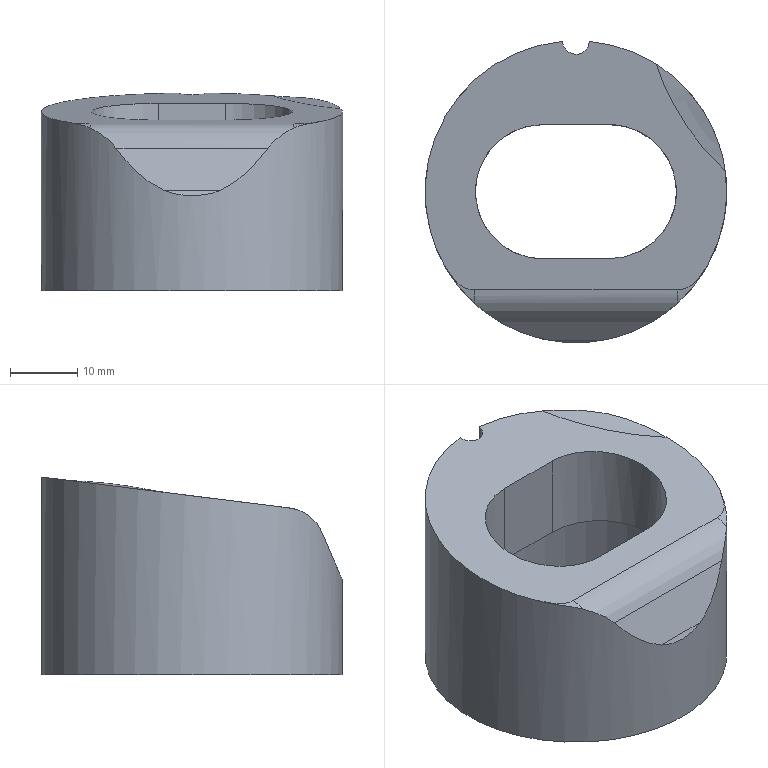Part | NX | features solid 2 | 1 solid | 18 faces | box 45 x 44.911 x 29.533 mm | volume 20669 mm3 | cylinder 9 | plane 6 | spline 3 | commonest cylinder face diameters 11.998 x2 20 x2 4 x1 12 x1 15 x1 36 x1
STEP:
#1=CARTESIAN_POINT('',(325.175,-191.134,24.41));
#2=VERTEX_POINT('',#1);
#3=CARTESIAN_POINT('',(325.178,-191.138,24.409));
#4=VERTEX_POINT('',#3);
#5=CARTESIAN_POINT('',(325.175,-191.134,24.41));
#6=CARTESIAN_POINT('',(325.176,-191.136,24.41));
#7=CARTESIAN_POINT('',(325.177,-191.137,24.41));
#8=CARTESIAN_POINT('',(325.178,-191.138,24.41));
#9=B_SPLINE_CURVE_WITH_KNOTS('',3,(#5,#6,#7,#8),.UNSPECIFIED.,.F.,.F.,(4,4),(0.6136,0.6142),.UNSPECIFIED.);
#10=EDGE_CURVE('',#2,#4,#9,.T.);
#11=ORIENTED_EDGE('',*,*,#10,.F.);
#12=CARTESIAN_POINT('',(343.002,-158.081,28.533));
#13=VERTEX_POINT('',#12);
#14=CARTESIAN_POINT('',(345.,-180.493,25.738));
#15=DIRECTION('',(0.,-0.1238,0.9923));
#16=DIRECTION('',(0.,0.9923,0.1238));
#17=AXIS2_PLACEMENT_3D('',#14,#15,#16);
#18=ELLIPSE('',#17,22.674,22.5);
#19=EDGE_CURVE('',#13,#2,#18,.T.);
#20=ORIENTED_EDGE('',*,*,#19,.F.);
#21=CARTESIAN_POINT('',(343.002,-158.081,-1.));
#22=VERTEX_POINT('',#21);
#23=CARTESIAN_POINT('',(343.002,-158.081,14.));
#24=DIRECTION('',(0.,0.,-1.));
#25=VECTOR('',#24,1000.);
#26=LINE('',#23,#25);
#27=EDGE_CURVE('',#22,#13,#26,.F.);
#28=ORIENTED_EDGE('',*,*,#27,.F.);
#29=CARTESIAN_POINT('',(346.998,-158.081,-1.));
#30=VERTEX_POINT('',#29);
#31=CARTESIAN_POINT('',(345.,-180.493,-1.));
#32=DIRECTION('',(0.,0.,-1.));
#33=DIRECTION('',(-1.,0.,0.));
#34=AXIS2_PLACEMENT_3D('',#31,#32,#33);
#35=CIRCLE('',#34,22.5);
#36=EDGE_CURVE('',#30,#22,#35,.T.);
#37=ORIENTED_EDGE('',*,*,#36,.F.);
#38=CARTESIAN_POINT('',(346.998,-158.081,28.533));
#39=VERTEX_POINT('',#38);
#40=CARTESIAN_POINT('',(346.998,-158.081,14.));
#41=DIRECTION('',(0.,0.,-1.));
#42=VECTOR('',#41,1000.);
#43=LINE('',#40,#42);
#44=EDGE_CURVE('',#39,#30,#43,.T.);
#45=ORIENTED_EDGE('',*,*,#44,.F.);
#46=CARTESIAN_POINT('',(357.006,-161.463,28.111));
#47=VERTEX_POINT('',#46);
#48=CARTESIAN_POINT('',(345.,-180.493,25.738));
#49=DIRECTION('',(0.,-0.1238,0.9923));
#50=DIRECTION('',(0.,0.9923,0.1238));
#51=AXIS2_PLACEMENT_3D('',#48,#49,#50);
#52=ELLIPSE('',#51,22.674,22.5);
#53=EDGE_CURVE('',#47,#39,#52,.T.);
#54=ORIENTED_EDGE('',*,*,#53,.F.);
#55=CARTESIAN_POINT('',(367.291,-177.436,26.119));
#56=VERTEX_POINT('',#55);
#57=CARTESIAN_POINT('',(367.291,-177.435,26.119));
#58=CARTESIAN_POINT('',(367.068,-175.804,26.322));
#59=CARTESIAN_POINT('',(366.286,-172.681,26.923));
#60=CARTESIAN_POINT('',(363.366,-166.778,27.871));
#61=CARTESIAN_POINT('',(359.804,-163.229,27.891));
#62=CARTESIAN_POINT('',(357.006,-161.463,28.111));
#63=B_SPLINE_CURVE_WITH_KNOTS('',3,(#57,#58,#59,#60,#61,#62),.UNSPECIFIED.,.F.,.F.,(4,1,1,4),(0.,0.004909,0.009818,0.01964),.UNSPECIFIED.);
#64=EDGE_CURVE('',#56,#47,#63,.T.);
#65=ORIENTED_EDGE('',*,*,#64,.F.);
#66=CARTESIAN_POINT('',(364.825,-191.134,24.41));
#67=VERTEX_POINT('',#66);
#68=CARTESIAN_POINT('',(345.,-180.493,25.738));
#69=DIRECTION('',(0.,-0.1238,0.9923));
#70=DIRECTION('',(0.,0.9923,0.1238));
#71=AXIS2_PLACEMENT_3D('',#68,#69,#70);
#72=ELLIPSE('',#71,22.674,22.5);
#73=EDGE_CURVE('',#67,#56,#72,.T.);
#74=ORIENTED_EDGE('',*,*,#73,.F.);
#75=CARTESIAN_POINT('',(364.822,-191.138,24.409));
#76=VERTEX_POINT('',#75);
#77=CARTESIAN_POINT('',(364.822,-191.138,24.41));
#78=CARTESIAN_POINT('',(364.823,-191.136,24.41));
#79=CARTESIAN_POINT('',(364.824,-191.135,24.41));
#80=CARTESIAN_POINT('',(364.825,-191.134,24.41));
#81=B_SPLINE_CURVE_WITH_KNOTS('',3,(#77,#78,#79,#80),.UNSPECIFIED.,.F.,.F.,(4,4),(0.3858,0.3865),.UNSPECIFIED.);
#82=EDGE_CURVE('',#76,#67,#81,.T.);
#83=ORIENTED_EDGE('',*,*,#82,.F.);
#84=CARTESIAN_POINT('',(363.388,-193.46,24.118));
#85=VERTEX_POINT('',#84);
#86=CARTESIAN_POINT('',(364.822,-191.138,24.409));
#87=CARTESIAN_POINT('',(364.392,-191.94,24.309));
#88=CARTESIAN_POINT('',(363.913,-192.714,24.211));
#89=CARTESIAN_POINT('',(363.388,-193.46,24.118));
#90=B_SPLINE_CURVE_WITH_KNOTS('',3,(#86,#87,#88,#89),.UNSPECIFIED.,.F.,.F.,(4,4),(0.0003971,0.003142),.UNSPECIFIED.);
#91=EDGE_CURVE('',#76,#85,#90,.T.);
#92=ORIENTED_EDGE('',*,*,#91,.T.);
#93=CARTESIAN_POINT('',(360.131,-197.145,23.293));
#94=VERTEX_POINT('',#93);
#95=CARTESIAN_POINT('',(363.388,-193.46,24.119));
#96=CARTESIAN_POINT('',(362.429,-194.818,23.95));
#97=CARTESIAN_POINT('',(361.302,-196.081,23.84));
#98=CARTESIAN_POINT('',(360.131,-197.145,23.293));
#99=B_SPLINE_CURVE_WITH_KNOTS('',3,(#95,#96,#97,#98),.UNSPECIFIED.,.F.,.F.,(4,4),(0.,0.005011),.UNSPECIFIED.);
#100=EDGE_CURVE('',#85,#94,#99,.T.);
#101=ORIENTED_EDGE('',*,*,#100,.T.);
#102=CARTESIAN_POINT('',(356.336,-199.928,20.3));
#103=VERTEX_POINT('',#102);
#104=CARTESIAN_POINT('',(360.131,-197.145,23.293));
#105=CARTESIAN_POINT('',(359.468,-197.747,22.984));
#106=CARTESIAN_POINT('',(358.149,-198.805,22.193));
#107=CARTESIAN_POINT('',(356.866,-199.619,21.027));
#108=CARTESIAN_POINT('',(356.336,-199.928,20.3));
#109=B_SPLINE_CURVE_WITH_KNOTS('',3,(#104,#105,#106,#107,#108),.UNSPECIFIED.,.F.,.F.,(4,1,4),(0.,0.002803,0.005605),.UNSPECIFIED.);
#110=EDGE_CURVE('',#94,#103,#109,.T.);
#111=ORIENTED_EDGE('',*,*,#110,.T.);
#112=CARTESIAN_POINT('',(349.112,-202.614,13.973));
#113=VERTEX_POINT('',#112);
#114=CARTESIAN_POINT('',(345.,-180.493,66.089));
#115=DIRECTION('',(0.,0.9205,-0.3907));
#116=DIRECTION('',(0.,0.3907,0.9205));
#117=AXIS2_PLACEMENT_3D('',#114,#115,#116);
#118=ELLIPSE('',#117,57.586,22.5);
#119=EDGE_CURVE('',#113,#103,#118,.F.);
#120=ORIENTED_EDGE('',*,*,#119,.F.);
#121=CARTESIAN_POINT('',(340.888,-202.614,13.973));
#122=VERTEX_POINT('',#121);
#123=CARTESIAN_POINT('',(340.888,-202.614,13.973));
#124=CARTESIAN_POINT('',(342.176,-202.853,13.409));
#125=CARTESIAN_POINT('',(344.991,-203.132,13.001));
#126=CARTESIAN_POINT('',(347.826,-202.853,13.41));
#127=CARTESIAN_POINT('',(349.112,-202.614,13.973));
#128=B_SPLINE_CURVE_WITH_KNOTS('',3,(#123,#124,#125,#126,#127),.UNSPECIFIED.,.F.,.F.,(4,1,4),(0.,0.004206,0.008413),.UNSPECIFIED.);
#129=EDGE_CURVE('',#122,#113,#128,.T.);
#130=ORIENTED_EDGE('',*,*,#129,.F.);
#131=CARTESIAN_POINT('',(333.664,-199.928,20.3));
#132=VERTEX_POINT('',#131);
#133=CARTESIAN_POINT('',(345.,-180.493,66.089));
#134=DIRECTION('',(0.,0.9205,-0.3907));
#135=DIRECTION('',(0.,0.3907,0.9205));
#136=AXIS2_PLACEMENT_3D('',#133,#134,#135);
#137=ELLIPSE('',#136,57.586,22.5);
#138=EDGE_CURVE('',#132,#122,#137,.F.);
#139=ORIENTED_EDGE('',*,*,#138,.F.);
#140=CARTESIAN_POINT('',(329.869,-197.145,23.293));
#141=VERTEX_POINT('',#140);
#142=CARTESIAN_POINT('',(333.664,-199.928,20.3));
#143=CARTESIAN_POINT('',(332.603,-199.309,21.757));
#144=CARTESIAN_POINT('',(331.194,-198.348,22.676));
#145=CARTESIAN_POINT('',(329.869,-197.145,23.293));
#146=B_SPLINE_CURVE_WITH_KNOTS('',3,(#142,#143,#144,#145),.UNSPECIFIED.,.F.,.F.,(4,4),(0.,0.00561),.UNSPECIFIED.);
#147=EDGE_CURVE('',#132,#141,#146,.T.);
#148=ORIENTED_EDGE('',*,*,#147,.T.);
#149=CARTESIAN_POINT('',(326.612,-193.46,24.119));
#150=VERTEX_POINT('',#149);
#151=CARTESIAN_POINT('',(329.869,-197.145,23.293));
#152=CARTESIAN_POINT('',(328.699,-196.082,23.839));
#153=CARTESIAN_POINT('',(327.57,-194.818,23.95));
#154=CARTESIAN_POINT('',(326.612,-193.46,24.119));
#155=B_SPLINE_CURVE_WITH_KNOTS('',3,(#151,#152,#153,#154),.UNSPECIFIED.,.F.,.F.,(4,4),(0.,0.005002),.UNSPECIFIED.);
#156=EDGE_CURVE('',#141,#150,#155,.T.);
#157=ORIENTED_EDGE('',*,*,#156,.T.);
#158=CARTESIAN_POINT('',(326.612,-193.46,24.119));
#159=CARTESIAN_POINT('',(326.087,-192.714,24.211));
#160=CARTESIAN_POINT('',(325.609,-191.94,24.309));
#161=CARTESIAN_POINT('',(325.178,-191.138,24.409));
#162=B_SPLINE_CURVE_WITH_KNOTS('',3,(#158,#159,#160,#161),.UNSPECIFIED.,.F.,.F.,(4,4),(0.0000426,0.002787),.UNSPECIFIED.);
#163=EDGE_CURVE('',#150,#4,#162,.T.);
#164=ORIENTED_EDGE('',*,*,#163,.T.);
#165=EDGE_LOOP('',(#11,#20,#28,#37,#45,#54,#65,#74,#83,#92,#101,#111,#120,#130,#139,#148,#157,#164));
#166=FACE_BOUND('',#165,.T.);
#167=CARTESIAN_POINT('',(345.,-180.493,-1.));
#168=DIRECTION('',(0.,0.,1.));
#169=DIRECTION('',(-1.,0.,0.));
#170=AXIS2_PLACEMENT_3D('',#167,#168,#169);
#171=CYLINDRICAL_SURFACE('',#170,22.5);
#172=ADVANCED_FACE('',(#166),#171,.T.);
#173=CARTESIAN_POINT('',(340.,-190.493,14.));
#174=VERTEX_POINT('',#173);
#175=CARTESIAN_POINT('',(340.,-190.493,24.49));
#176=VERTEX_POINT('',#175);
#177=CARTESIAN_POINT('',(340.,-190.493,-251.));
#178=DIRECTION('',(0.,0.,1.));
#179=VECTOR('',#178,1000.);
#180=LINE('',#177,#179);
#181=EDGE_CURVE('',#174,#176,#180,.T.);
#182=ORIENTED_EDGE('',*,*,#181,.T.);
#183=CARTESIAN_POINT('',(350.,-190.493,24.49));
#184=VERTEX_POINT('',#183);
#185=CARTESIAN_POINT('',(340.,-190.493,24.49));
#186=DIRECTION('',(1.,0.,0.));
#187=VECTOR('',#186,1000.);
#188=LINE('',#185,#187);
#189=EDGE_CURVE('',#176,#184,#188,.T.);
#190=ORIENTED_EDGE('',*,*,#189,.T.);
#191=CARTESIAN_POINT('',(350.,-190.493,14.));
#192=VERTEX_POINT('',#191);
#193=CARTESIAN_POINT('',(350.,-190.493,-251.));
#194=DIRECTION('',(0.,0.,1.));
#195=VECTOR('',#194,1000.);
#196=LINE('',#193,#195);
#197=EDGE_CURVE('',#192,#184,#196,.T.);
#198=ORIENTED_EDGE('',*,*,#197,.F.);
#199=CARTESIAN_POINT('',(340.,-190.493,14.));
#200=DIRECTION('',(-1.,0.,0.));
#201=VECTOR('',#200,1000.);
#202=LINE('',#199,#201);
#203=EDGE_CURVE('',#192,#174,#202,.T.);
#204=ORIENTED_EDGE('',*,*,#203,.T.);
#205=EDGE_LOOP('',(#182,#190,#198,#204));
#206=FACE_BOUND('',#205,.T.);
#207=CARTESIAN_POINT('',(340.,-190.493,-251.));
#208=DIRECTION('',(0.,1.,0.));
#209=DIRECTION('',(0.,0.,1.));
#210=AXIS2_PLACEMENT_3D('',#207,#208,#209);
#211=PLANE('',#210);
#212=ADVANCED_FACE('',(#206),#211,.T.);
#213=CARTESIAN_POINT('',(359.96,-181.391,25.625));
#214=VERTEX_POINT('',#213);
#215=CARTESIAN_POINT('',(350.,-180.493,25.738));
#216=DIRECTION('',(0.,-0.1238,0.9923));
#217=DIRECTION('',(0.,0.9923,0.1238));
#218=AXIS2_PLACEMENT_3D('',#215,#216,#217);
#219=ELLIPSE('',#218,10.078,10.);
#220=EDGE_CURVE('',#214,#184,#219,.F.);
#221=ORIENTED_EDGE('',*,*,#220,.F.);
#222=CARTESIAN_POINT('',(359.958,-179.573,25.852));
#223=VERTEX_POINT('',#222);
#224=CARTESIAN_POINT('',(359.958,-179.573,25.852));
#225=CARTESIAN_POINT('',(360.014,-180.18,25.777));
#226=CARTESIAN_POINT('',(360.014,-180.789,25.701));
#227=CARTESIAN_POINT('',(359.96,-181.391,25.625));
#228=B_SPLINE_CURVE_WITH_KNOTS('',3,(#224,#225,#226,#227),.UNSPECIFIED.,.F.,.F.,(4,4),(0.4706,0.5289),.UNSPECIFIED.);
#229=EDGE_CURVE('',#223,#214,#228,.T.);
#230=ORIENTED_EDGE('',*,*,#229,.F.);
#231=CARTESIAN_POINT('',(350.,-170.493,26.985));
#232=VERTEX_POINT('',#231);
#233=CARTESIAN_POINT('',(350.,-180.493,25.738));
#234=DIRECTION('',(0.,-0.1238,0.9923));
#235=DIRECTION('',(0.,0.9923,0.1238));
#236=AXIS2_PLACEMENT_3D('',#233,#234,#235);
#237=ELLIPSE('',#236,10.078,10.);
#238=EDGE_CURVE('',#232,#223,#237,.F.);
#239=ORIENTED_EDGE('',*,*,#238,.F.);
#240=CARTESIAN_POINT('',(350.,-170.493,14.));
#241=VERTEX_POINT('',#240);
#242=CARTESIAN_POINT('',(350.,-170.493,-251.));
#243=DIRECTION('',(0.,0.,1.));
#244=VECTOR('',#243,1000.);
#245=LINE('',#242,#244);
#246=EDGE_CURVE('',#241,#232,#245,.T.);
#247=ORIENTED_EDGE('',*,*,#246,.F.);
#248=CARTESIAN_POINT('',(350.,-180.493,14.));
#249=DIRECTION('',(0.,0.,-1.));
#250=DIRECTION('',(-1.,0.,0.));
#251=AXIS2_PLACEMENT_3D('',#248,#249,#250);
#252=CIRCLE('',#251,10.);
#253=EDGE_CURVE('',#192,#241,#252,.F.);
#254=ORIENTED_EDGE('',*,*,#253,.F.);
#255=ORIENTED_EDGE('',*,*,#197,.T.);
#256=EDGE_LOOP('',(#221,#230,#239,#247,#254,#255));
#257=FACE_BOUND('',#256,.T.);
#258=CARTESIAN_POINT('',(350.,-180.493,-251.));
#259=DIRECTION('',(0.,0.,1.));
#260=DIRECTION('',(-1.,0.,0.));
#261=AXIS2_PLACEMENT_3D('',#258,#259,#260);
#262=CYLINDRICAL_SURFACE('',#261,10.);
#263=ADVANCED_FACE('',(#257),#262,.F.);
#264=CARTESIAN_POINT('',(340.,-170.493,26.985));
#265=VERTEX_POINT('',#264);
#266=CARTESIAN_POINT('',(340.,-170.493,26.985));
#267=DIRECTION('',(1.,0.,0.));
#268=VECTOR('',#267,1000.);
#269=LINE('',#266,#268);
#270=EDGE_CURVE('',#265,#232,#269,.T.);
#271=ORIENTED_EDGE('',*,*,#270,.F.);
#272=CARTESIAN_POINT('',(340.,-170.493,14.));
#273=VERTEX_POINT('',#272);
#274=CARTESIAN_POINT('',(340.,-170.493,-251.));
#275=DIRECTION('',(0.,0.,1.));
#276=VECTOR('',#275,1000.);
#277=LINE('',#274,#276);
#278=EDGE_CURVE('',#273,#265,#277,.T.);
#279=ORIENTED_EDGE('',*,*,#278,.F.);
#280=CARTESIAN_POINT('',(340.,-170.493,14.));
#281=DIRECTION('',(-1.,0.,0.));
#282=VECTOR('',#281,1000.);
#283=LINE('',#280,#282);
#284=EDGE_CURVE('',#241,#273,#283,.T.);
#285=ORIENTED_EDGE('',*,*,#284,.F.);
#286=ORIENTED_EDGE('',*,*,#246,.T.);
#287=EDGE_LOOP('',(#271,#279,#285,#286));
#288=FACE_BOUND('',#287,.T.);
#289=CARTESIAN_POINT('',(340.,-170.493,-251.));
#290=DIRECTION('',(0.,1.,0.));
#291=DIRECTION('',(0.,0.,1.));
#292=AXIS2_PLACEMENT_3D('',#289,#290,#291);
#293=PLANE('',#292);
#294=ADVANCED_FACE('',(#288),#293,.F.);
#295=CARTESIAN_POINT('',(330.042,-181.411,25.623));
#296=VERTEX_POINT('',#295);
#297=CARTESIAN_POINT('',(340.,-180.493,25.738));
#298=DIRECTION('',(0.,-0.1238,0.9923));
#299=DIRECTION('',(0.,0.9923,0.1238));
#300=AXIS2_PLACEMENT_3D('',#297,#298,#299);
#301=ELLIPSE('',#300,10.078,10.);
#302=EDGE_CURVE('',#176,#296,#301,.F.);
#303=ORIENTED_EDGE('',*,*,#302,.F.);
#304=ORIENTED_EDGE('',*,*,#181,.F.);
#305=CARTESIAN_POINT('',(340.,-180.493,14.));
#306=DIRECTION('',(0.,0.,-1.));
#307=DIRECTION('',(-1.,0.,0.));
#308=AXIS2_PLACEMENT_3D('',#305,#306,#307);
#309=CIRCLE('',#308,10.);
#310=EDGE_CURVE('',#273,#174,#309,.F.);
#311=ORIENTED_EDGE('',*,*,#310,.F.);
#312=ORIENTED_EDGE('',*,*,#278,.T.);
#313=CARTESIAN_POINT('',(330.04,-179.594,25.85));
#314=VERTEX_POINT('',#313);
#315=CARTESIAN_POINT('',(340.,-180.493,25.738));
#316=DIRECTION('',(0.,-0.1238,0.9923));
#317=DIRECTION('',(0.,0.9923,0.1238));
#318=AXIS2_PLACEMENT_3D('',#315,#316,#317);
#319=ELLIPSE('',#318,10.078,10.);
#320=EDGE_CURVE('',#314,#265,#319,.F.);
#321=ORIENTED_EDGE('',*,*,#320,.F.);
#322=CARTESIAN_POINT('',(330.042,-181.411,25.623));
#323=CARTESIAN_POINT('',(329.986,-180.804,25.699));
#324=CARTESIAN_POINT('',(329.986,-180.196,25.775));
#325=CARTESIAN_POINT('',(330.04,-179.594,25.85));
#326=B_SPLINE_CURVE_WITH_KNOTS('',3,(#322,#323,#324,#325),.UNSPECIFIED.,.F.,.F.,(4,4),(0.4706,0.5289),.UNSPECIFIED.);
#327=EDGE_CURVE('',#296,#314,#326,.T.);
#328=ORIENTED_EDGE('',*,*,#327,.F.);
#329=EDGE_LOOP('',(#303,#304,#311,#312,#321,#328));
#330=FACE_BOUND('',#329,.T.);
#331=CARTESIAN_POINT('',(340.,-180.493,-251.));
#332=DIRECTION('',(0.,0.,1.));
#333=DIRECTION('',(-1.,0.,0.));
#334=AXIS2_PLACEMENT_3D('',#331,#332,#333);
#335=CYLINDRICAL_SURFACE('',#334,10.);
#336=ADVANCED_FACE('',(#330),#335,.F.);
#337=CARTESIAN_POINT('',(345.,-157.993,28.544));
#338=DIRECTION('',(0.,-0.1238,0.9923));
#339=DIRECTION('',(0.,-0.9923,-0.1238));
#340=AXIS2_PLACEMENT_3D('',#337,#338,#339);
#341=ELLIPSE('',#340,2.016,2.);
#342=EDGE_CURVE('',#39,#13,#341,.F.);
#343=ORIENTED_EDGE('',*,*,#342,.F.);
#344=ORIENTED_EDGE('',*,*,#44,.T.);
#345=CARTESIAN_POINT('',(345.,-157.993,-1.));
#346=DIRECTION('',(0.,0.,-1.));
#347=DIRECTION('',(0.,-1.,0.));
#348=AXIS2_PLACEMENT_3D('',#345,#346,#347);
#349=CIRCLE('',#348,2.);
#350=EDGE_CURVE('',#30,#22,#349,.T.);
#351=ORIENTED_EDGE('',*,*,#350,.T.);
#352=ORIENTED_EDGE('',*,*,#27,.T.);
#353=EDGE_LOOP('',(#343,#344,#351,#352));
#354=FACE_BOUND('',#353,.T.);
#355=CARTESIAN_POINT('',(345.,-157.993,29.));
#356=DIRECTION('',(0.,0.,-1.));
#357=DIRECTION('',(0.,1.,0.));
#358=AXIS2_PLACEMENT_3D('',#355,#356,#357);
#359=CYLINDRICAL_SURFACE('',#358,2.);
#360=ADVANCED_FACE('',(#354),#359,.F.);
#361=ORIENTED_EDGE('',*,*,#36,.T.);
#362=ORIENTED_EDGE('',*,*,#350,.F.);
#363=EDGE_LOOP('',(#361,#362));
#364=FACE_BOUND('',#363,.T.);
#365=CARTESIAN_POINT('',(327.,-180.493,-1.));
#366=VERTEX_POINT('',#365);
#367=CARTESIAN_POINT('',(345.,-180.493,-1.));
#368=DIRECTION('',(0.,0.,-1.));
#369=DIRECTION('',(-1.,0.,0.));
#370=AXIS2_PLACEMENT_3D('',#367,#368,#369);
#371=CIRCLE('',#370,18.);
#372=EDGE_CURVE('',#366,#366,#371,.F.);
#373=ORIENTED_EDGE('',*,*,#372,.T.);
#374=EDGE_LOOP('',(#373));
#375=FACE_BOUND('',#374,.T.);
#376=CARTESIAN_POINT('',(345.,-180.493,-1.));
#377=DIRECTION('',(0.,0.,1.));
#378=DIRECTION('',(-1.,0.,0.));
#379=AXIS2_PLACEMENT_3D('',#376,#377,#378);
#380=PLANE('',#379);
#381=ADVANCED_FACE('',(#364,#375),#380,.F.);
#382=CARTESIAN_POINT('',(327.,-180.493,14.));
#383=VERTEX_POINT('',#382);
#384=CARTESIAN_POINT('',(345.,-180.493,14.));
#385=DIRECTION('',(0.,0.,-1.));
#386=DIRECTION('',(-1.,0.,0.));
#387=AXIS2_PLACEMENT_3D('',#384,#385,#386);
#388=CIRCLE('',#387,18.);
#389=EDGE_CURVE('',#383,#383,#388,.T.);
#390=ORIENTED_EDGE('',*,*,#389,.F.);
#391=EDGE_LOOP('',(#390));
#392=FACE_BOUND('',#391,.T.);
#393=ORIENTED_EDGE('',*,*,#372,.F.);
#394=EDGE_LOOP('',(#393));
#395=FACE_BOUND('',#394,.T.);
#396=CARTESIAN_POINT('',(345.,-180.493,21.));
#397=DIRECTION('',(0.,0.,-1.));
#398=DIRECTION('',(1.,0.,0.));
#399=AXIS2_PLACEMENT_3D('',#396,#397,#398);
#400=CYLINDRICAL_SURFACE('',#399,18.);
#401=ADVANCED_FACE('',(#392,#395),#400,.F.);
#402=ORIENTED_EDGE('',*,*,#203,.F.);
#403=ORIENTED_EDGE('',*,*,#253,.T.);
#404=ORIENTED_EDGE('',*,*,#284,.T.);
#405=ORIENTED_EDGE('',*,*,#310,.T.);
#406=EDGE_LOOP('',(#402,#403,#404,#405));
#407=FACE_BOUND('',#406,.T.);
#408=ORIENTED_EDGE('',*,*,#389,.T.);
#409=EDGE_LOOP('',(#408));
#410=FACE_BOUND('',#409,.T.);
#411=CARTESIAN_POINT('',(345.,-180.493,14.));
#412=DIRECTION('',(0.,0.,1.));
#413=DIRECTION('',(-1.,0.,0.));
#414=AXIS2_PLACEMENT_3D('',#411,#412,#413);
#415=PLANE('',#414);
#416=ADVANCED_FACE('',(#407,#410),#415,.F.);
#417=ORIENTED_EDGE('',*,*,#73,.T.);
#418=CARTESIAN_POINT('',(367.29,-177.439,26.119));
#419=CARTESIAN_POINT('',(362.583,-173.071,26.663));
#420=CARTESIAN_POINT('',(358.98,-167.562,27.351));
#421=CARTESIAN_POINT('',(357.004,-161.463,28.111));
#422=B_SPLINE_CURVE_WITH_KNOTS('',3,(#418,#419,#420,#421),.UNSPECIFIED.,.F.,.F.,(4,4),(0.1646,0.5757),.UNSPECIFIED.);
#423=EDGE_CURVE('',#56,#47,#422,.T.);
#424=ORIENTED_EDGE('',*,*,#423,.T.);
#425=ORIENTED_EDGE('',*,*,#53,.T.);
#426=ORIENTED_EDGE('',*,*,#342,.T.);
#427=ORIENTED_EDGE('',*,*,#19,.T.);
#428=ORIENTED_EDGE('',*,*,#10,.T.);
#429=CARTESIAN_POINT('',(326.718,-193.389,24.129));
#430=VERTEX_POINT('',#429);
#431=CARTESIAN_POINT('',(325.178,-191.138,24.41));
#432=CARTESIAN_POINT('',(325.691,-191.888,24.316));
#433=CARTESIAN_POINT('',(326.205,-192.639,24.222));
#434=CARTESIAN_POINT('',(326.718,-193.389,24.129));
#435=B_SPLINE_CURVE_WITH_KNOTS('',3,(#431,#432,#433,#434),.UNSPECIFIED.,.F.,.F.,(4,4),(0.6142,1.),.UNSPECIFIED.);
#436=EDGE_CURVE('',#4,#430,#435,.T.);
#437=ORIENTED_EDGE('',*,*,#436,.T.);
#438=CARTESIAN_POINT('',(329.869,-195.148,23.909));
#439=VERTEX_POINT('',#438);
#440=CARTESIAN_POINT('',(326.718,-193.389,24.129));
#441=CARTESIAN_POINT('',(326.837,-193.558,24.108));
#442=CARTESIAN_POINT('',(326.981,-193.748,24.084));
#443=CARTESIAN_POINT('',(327.433,-194.232,24.024));
#444=CARTESIAN_POINT('',(328.051,-194.689,23.967));
#445=CARTESIAN_POINT('',(328.787,-195.002,23.928));
#446=CARTESIAN_POINT('',(329.314,-195.113,23.914));
#447=CARTESIAN_POINT('',(329.645,-195.141,23.91));
#448=CARTESIAN_POINT('',(329.764,-195.145,23.91));
#449=CARTESIAN_POINT('',(329.869,-195.148,23.909));
#450=B_SPLINE_CURVE_WITH_KNOTS('',3,(#440,#441,#442,#443,#444,#445,#446,#447,#448,#449),.UNSPECIFIED.,.F.,.F.,(4,1,1,1,1,1,1,4),(0.,0.125,0.25,0.5,0.75,0.875,0.9375,1.),.UNSPECIFIED.);
#451=EDGE_CURVE('',#430,#439,#450,.T.);
#452=ORIENTED_EDGE('',*,*,#451,.T.);
#453=CARTESIAN_POINT('',(360.131,-195.148,23.909));
#454=VERTEX_POINT('',#453);
#455=CARTESIAN_POINT('',(329.869,-195.148,23.909));
#456=CARTESIAN_POINT('',(339.956,-195.148,23.909));
#457=CARTESIAN_POINT('',(350.044,-195.148,23.909));
#458=CARTESIAN_POINT('',(360.131,-195.148,23.909));
#459=B_SPLINE_CURVE_WITH_KNOTS('',3,(#455,#456,#457,#458),.UNSPECIFIED.,.F.,.F.,(4,4),(0.,1.),.UNSPECIFIED.);
#460=EDGE_CURVE('',#439,#454,#459,.T.);
#461=ORIENTED_EDGE('',*,*,#460,.T.);
#462=CARTESIAN_POINT('',(363.281,-193.389,24.129));
#463=VERTEX_POINT('',#462);
#464=CARTESIAN_POINT('',(360.131,-195.148,23.909));
#465=CARTESIAN_POINT('',(360.339,-195.145,23.91));
#466=CARTESIAN_POINT('',(360.578,-195.129,23.912));
#467=CARTESIAN_POINT('',(361.23,-195.003,23.927));
#468=CARTESIAN_POINT('',(361.942,-194.69,23.966));
#469=CARTESIAN_POINT('',(362.566,-194.233,24.023));
#470=CARTESIAN_POINT('',(363.019,-193.75,24.084));
#471=CARTESIAN_POINT('',(363.159,-193.56,24.107));
#472=CARTESIAN_POINT('',(363.281,-193.39,24.129));
#473=B_SPLINE_CURVE_WITH_KNOTS('',3,(#464,#465,#466,#467,#468,#469,#470,#471,#472),.UNSPECIFIED.,.F.,.F.,(4,1,1,1,1,1,4),(0.,0.125,0.25,0.5,0.75,0.875,1.),.UNSPECIFIED.);
#474=EDGE_CURVE('',#454,#463,#473,.T.);
#475=ORIENTED_EDGE('',*,*,#474,.T.);
#476=CARTESIAN_POINT('',(363.282,-193.389,24.129));
#477=CARTESIAN_POINT('',(363.795,-192.638,24.222));
#478=CARTESIAN_POINT('',(364.309,-191.888,24.316));
#479=CARTESIAN_POINT('',(364.822,-191.138,24.41));
#480=B_SPLINE_CURVE_WITH_KNOTS('',3,(#476,#477,#478,#479),.UNSPECIFIED.,.F.,.F.,(4,4),(0.,0.3858),.UNSPECIFIED.);
#481=EDGE_CURVE('',#463,#76,#480,.T.);
#482=ORIENTED_EDGE('',*,*,#481,.T.);
#483=ORIENTED_EDGE('',*,*,#82,.T.);
#484=EDGE_LOOP('',(#417,#424,#425,#426,#427,#428,#437,#452,#461,#475,#482,#483));
#485=FACE_BOUND('',#484,.T.);
#486=ORIENTED_EDGE('',*,*,#229,.T.);
#487=ORIENTED_EDGE('',*,*,#220,.T.);
#488=ORIENTED_EDGE('',*,*,#189,.F.);
#489=ORIENTED_EDGE('',*,*,#302,.T.);
#490=ORIENTED_EDGE('',*,*,#327,.T.);
#491=ORIENTED_EDGE('',*,*,#320,.T.);
#492=ORIENTED_EDGE('',*,*,#270,.T.);
#493=ORIENTED_EDGE('',*,*,#238,.T.);
#494=EDGE_LOOP('',(#486,#487,#488,#489,#490,#491,#492,#493));
#495=FACE_BOUND('',#494,.T.);
#496=CARTESIAN_POINT('',(300.,-92.289,36.741));
#497=DIRECTION('',(0.,-0.1238,0.9923));
#498=DIRECTION('',(0.,0.9923,0.1238));
#499=AXIS2_PLACEMENT_3D('',#496,#497,#498);
#500=PLANE('',#499);
#501=ADVANCED_FACE('',(#485,#495),#500,.T.);
#502=CARTESIAN_POINT('',(349.112,-202.614,13.973));
#503=CARTESIAN_POINT('',(346.371,-202.614,13.973));
#504=CARTESIAN_POINT('',(343.629,-202.614,13.973));
#505=CARTESIAN_POINT('',(340.888,-202.614,13.973));
#506=B_SPLINE_CURVE_WITH_KNOTS('',3,(#502,#503,#504,#505),.UNSPECIFIED.,.F.,.F.,(4,4),(0.364,0.636),.UNSPECIFIED.);
#507=EDGE_CURVE('',#113,#122,#506,.T.);
#508=ORIENTED_EDGE('',*,*,#507,.T.);
#509=ORIENTED_EDGE('',*,*,#129,.T.);
#510=EDGE_LOOP('',(#508,#509));
#511=FACE_BOUND('',#510,.T.);
#512=CARTESIAN_POINT('',(354.069,-209.517,16.904));
#513=DIRECTION('',(1.,0.,0.));
#514=DIRECTION('',(0.,1.,0.));
#515=AXIS2_PLACEMENT_3D('',#512,#513,#514);
#516=CYLINDRICAL_SURFACE('',#515,7.5);
#517=ADVANCED_FACE('',(#511),#516,.F.);
#518=CARTESIAN_POINT('',(333.664,-199.928,20.3));
#519=CARTESIAN_POINT('',(341.221,-199.928,20.3));
#520=CARTESIAN_POINT('',(348.779,-199.928,20.3));
#521=CARTESIAN_POINT('',(356.336,-199.928,20.3));
#522=B_SPLINE_CURVE_WITH_KNOTS('',3,(#518,#519,#520,#521),.UNSPECIFIED.,.F.,.F.,(4,4),(0.1254,0.8746),.UNSPECIFIED.);
#523=EDGE_CURVE('',#132,#103,#522,.T.);
#524=ORIENTED_EDGE('',*,*,#523,.F.);
#525=ORIENTED_EDGE('',*,*,#138,.T.);
#526=ORIENTED_EDGE('',*,*,#507,.F.);
#527=ORIENTED_EDGE('',*,*,#119,.T.);
#528=EDGE_LOOP('',(#524,#525,#526,#527));
#529=FACE_BOUND('',#528,.T.);
#530=CARTESIAN_POINT('',(360.312,-199.928,20.3));
#531=DIRECTION('',(0.,0.9205,-0.3907));
#532=DIRECTION('',(0.,-0.3907,-0.9205));
#533=AXIS2_PLACEMENT_3D('',#530,#531,#532);
#534=PLANE('',#533);
#535=ADVANCED_FACE('',(#529),#534,.F.);
#536=ORIENTED_EDGE('',*,*,#423,.F.);
#537=ORIENTED_EDGE('',*,*,#64,.T.);
#538=EDGE_LOOP('',(#536,#537));
#539=FACE_BOUND('',#538,.T.);
#540=CARTESIAN_POINT('',(370.014,-175.954,26.616));
#541=CARTESIAN_POINT('',(368.713,-174.589,26.802));
#542=CARTESIAN_POINT('',(367.472,-173.09,27.004));
#543=CARTESIAN_POINT('',(365.774,-170.65,27.329));
#544=CARTESIAN_POINT('',(365.244,-169.821,27.439));
#545=CARTESIAN_POINT('',(364.24,-168.096,27.667));
#546=CARTESIAN_POINT('',(363.737,-167.132,27.794));
#547=CARTESIAN_POINT('',(362.629,-164.805,28.099));
#548=CARTESIAN_POINT('',(361.893,-162.979,28.337));
#549=CARTESIAN_POINT('',(361.269,-160.795,28.619));
#550=CARTESIAN_POINT('',(361.257,-160.756,28.624));
#551=CARTESIAN_POINT('',(361.246,-160.717,28.63));
#552=CARTESIAN_POINT('',(368.706,-176.704,26.21));
#553=CARTESIAN_POINT('',(367.301,-175.326,26.382));
#554=CARTESIAN_POINT('',(365.955,-173.8,26.572));
#555=CARTESIAN_POINT('',(364.106,-171.299,26.884));
#556=CARTESIAN_POINT('',(363.527,-170.446,26.991));
#557=CARTESIAN_POINT('',(362.428,-168.667,27.213));
#558=CARTESIAN_POINT('',(361.877,-167.669,27.337));
#559=CARTESIAN_POINT('',(360.659,-165.256,27.638));
#560=CARTESIAN_POINT('',(359.846,-163.358,27.875));
#561=CARTESIAN_POINT('',(359.151,-161.078,28.159));
#562=CARTESIAN_POINT('',(359.138,-161.038,28.165));
#563=CARTESIAN_POINT('',(359.126,-160.997,28.17));
#564=CARTESIAN_POINT('',(367.372,-177.509,26.11));
#565=CARTESIAN_POINT('',(365.861,-176.119,26.283));
#566=CARTESIAN_POINT('',(364.408,-174.568,26.477));
#567=CARTESIAN_POINT('',(362.404,-172.005,26.796));
#568=CARTESIAN_POINT('',(361.776,-171.13,26.906));
#569=CARTESIAN_POINT('',(360.581,-169.296,27.134));
#570=CARTESIAN_POINT('',(359.981,-168.266,27.263));
#571=CARTESIAN_POINT('',(358.651,-165.767,27.574));
#572=CARTESIAN_POINT('',(357.76,-163.796,27.82));
#573=CARTESIAN_POINT('',(356.992,-161.42,28.117));
#574=CARTESIAN_POINT('',(356.978,-161.378,28.122));
#575=CARTESIAN_POINT('',(356.965,-161.335,28.127));
#576=(BOUNDED_SURFACE()B_SPLINE_SURFACE(2,3,((#540,#541,#542,#543,#544,#545,#546,#547,#548,#549,#550,#551),(#552,#553,#554,#555,#556,#557,#558,#559,#560,#561,#562,#563),(#564,#565,#566,#567,#568,#569,#570,#571,#572,#573,#574,#575)),.UNSPECIFIED.,.F.,.F.,.F.)B_SPLINE_SURFACE_WITH_KNOTS((3,3),(4,2,2,2,2,4),(0.8161,1.),(0.5603,0.625,0.6562,0.6875,0.75,0.7511),.UNSPECIFIED.)GEOMETRIC_REPRESENTATION_ITEM()RATIONAL_B_SPLINE_SURFACE(((0.9544,0.9548,0.9552,0.9557,0.9558,0.9562,0.9563,0.9567,0.9569,0.9571,0.9571,0.9571),(0.9721,0.9723,0.9725,0.9729,0.973,0.9731,0.9732,0.9734,0.9736,0.9737,0.9737,0.9737),(1.,1.,1.,1.,1.,1.,1.,1.,1.,1.,1.,1.)))REPRESENTATION_ITEM('')SURFACE());
#577=ADVANCED_FACE('',(#539),#576,.F.);
#578=ORIENTED_EDGE('',*,*,#163,.F.);
#579=CARTESIAN_POINT('',(326.612,-193.46,24.119));
#580=CARTESIAN_POINT('',(326.648,-193.436,24.122));
#581=CARTESIAN_POINT('',(326.683,-193.413,24.126));
#582=CARTESIAN_POINT('',(326.718,-193.389,24.129));
#583=B_SPLINE_CURVE_WITH_KNOTS('',3,(#579,#580,#581,#582),.UNSPECIFIED.,.F.,.F.,(4,4),(0.9881,1.),.UNSPECIFIED.);
#584=EDGE_CURVE('',#430,#150,#583,.F.);
#585=ORIENTED_EDGE('',*,*,#584,.F.);
#586=ORIENTED_EDGE('',*,*,#436,.F.);
#587=EDGE_LOOP('',(#578,#585,#586));
#588=FACE_BOUND('',#587,.T.);
#589=CARTESIAN_POINT('',(325.92,-191.479,18.322));
#590=DIRECTION('',(0.5619,-0.8208,-0.1023));
#591=DIRECTION('',(0.8252,0.5649,0.));
#592=AXIS2_PLACEMENT_3D('',#589,#590,#591);
#593=CYLINDRICAL_SURFACE('',#592,5.999);
#594=ADVANCED_FACE('',(#588),#593,.T.);
#595=ORIENTED_EDGE('',*,*,#156,.F.);
#596=CARTESIAN_POINT('',(329.869,-195.148,23.909));
#597=CARTESIAN_POINT('',(329.869,-195.843,23.823));
#598=CARTESIAN_POINT('',(329.869,-196.522,23.613));
#599=CARTESIAN_POINT('',(329.869,-197.145,23.293));
#600=B_SPLINE_CURVE_WITH_KNOTS('',3,(#596,#597,#598,#599),.UNSPECIFIED.,.F.,.F.,(4,4),(0.,0.335),.UNSPECIFIED.);
#601=EDGE_CURVE('',#439,#141,#600,.T.);
#602=ORIENTED_EDGE('',*,*,#601,.F.);
#603=ORIENTED_EDGE('',*,*,#451,.F.);
#604=ORIENTED_EDGE('',*,*,#584,.T.);
#605=EDGE_LOOP('',(#595,#602,#603,#604));
#606=FACE_BOUND('',#605,.T.);
#607=CARTESIAN_POINT('',(329.869,-195.148,23.909));
#608=CARTESIAN_POINT('',(329.869,-196.208,23.777));
#609=CARTESIAN_POINT('',(329.869,-197.157,23.287));
#610=CARTESIAN_POINT('',(329.552,-195.148,23.909));
#611=CARTESIAN_POINT('',(329.455,-196.208,23.777));
#612=CARTESIAN_POINT('',(329.363,-197.157,23.287));
#613=CARTESIAN_POINT('',(329.243,-195.105,23.915));
#614=CARTESIAN_POINT('',(329.05,-196.158,23.783));
#615=CARTESIAN_POINT('',(328.869,-197.099,23.291));
#616=CARTESIAN_POINT('',(328.866,-195.002,23.928));
#617=CARTESIAN_POINT('',(328.554,-196.036,23.799));
#618=CARTESIAN_POINT('',(328.262,-196.957,23.299));
#619=CARTESIAN_POINT('',(328.791,-194.979,23.93));
#620=CARTESIAN_POINT('',(328.455,-196.008,23.802));
#621=CARTESIAN_POINT('',(328.141,-196.925,23.301));
#622=CARTESIAN_POINT('',(328.642,-194.927,23.937));
#623=CARTESIAN_POINT('',(328.259,-195.948,23.81));
#624=CARTESIAN_POINT('',(327.901,-196.854,23.305));
#625=CARTESIAN_POINT('',(328.568,-194.899,23.94));
#626=CARTESIAN_POINT('',(328.161,-195.914,23.814));
#627=CARTESIAN_POINT('',(327.781,-196.815,23.308));
#628=CARTESIAN_POINT('',(328.351,-194.808,23.952));
#629=CARTESIAN_POINT('',(327.874,-195.807,23.827));
#630=CARTESIAN_POINT('',(327.43,-196.689,23.315));
#631=CARTESIAN_POINT('',(328.211,-194.739,23.96));
#632=CARTESIAN_POINT('',(327.689,-195.724,23.837));
#633=CARTESIAN_POINT('',(327.202,-196.593,23.321));
#634=CARTESIAN_POINT('',(327.94,-194.583,23.98));
#635=CARTESIAN_POINT('',(327.329,-195.54,23.86));
#636=CARTESIAN_POINT('',(326.76,-196.377,23.334));
#637=CARTESIAN_POINT('',(327.81,-194.497,23.99));
#638=CARTESIAN_POINT('',(327.154,-195.437,23.873));
#639=CARTESIAN_POINT('',(326.545,-196.258,23.341));
#640=CARTESIAN_POINT('',(327.621,-194.356,24.008));
#641=CARTESIAN_POINT('',(326.9,-195.269,23.894));
#642=CARTESIAN_POINT('',(326.231,-196.061,23.353));
#643=CARTESIAN_POINT('',(327.559,-194.307,24.014));
#644=CARTESIAN_POINT('',(326.816,-195.21,23.902));
#645=CARTESIAN_POINT('',(326.128,-195.992,23.358));
#646=CARTESIAN_POINT('',(327.439,-194.206,24.027));
#647=CARTESIAN_POINT('',(326.654,-195.09,23.917));
#648=CARTESIAN_POINT('',(325.927,-195.851,23.366));
#649=CARTESIAN_POINT('',(327.381,-194.154,24.033));
#650=CARTESIAN_POINT('',(326.574,-195.027,23.924));
#651=CARTESIAN_POINT('',(325.829,-195.778,23.371));
#652=CARTESIAN_POINT('',(327.097,-193.886,24.067));
#653=CARTESIAN_POINT('',(326.188,-194.707,23.964));
#654=CARTESIAN_POINT('',(325.35,-195.401,23.393));
#655=CARTESIAN_POINT('',(326.896,-193.648,24.096));
#656=CARTESIAN_POINT('',(325.908,-194.42,24.));
#657=CARTESIAN_POINT('',(325.002,-195.065,23.413));
#658=CARTESIAN_POINT('',(326.718,-193.389,24.129));
#659=CARTESIAN_POINT('',(325.655,-194.105,24.039));
#660=CARTESIAN_POINT('',(324.685,-194.693,23.436));
#661=(BOUNDED_SURFACE()B_SPLINE_SURFACE(3,2,((#607,#608,#609),(#610,#611,#612),(#613,#614,#615),(#616,#617,#618),(#619,#620,#621),(#622,#623,#624),(#625,#626,#627),(#628,#629,#630),(#631,#632,#633),(#634,#635,#636),(#637,#638,#639),(#640,#641,#642),(#643,#644,#645),(#646,#647,#648),(#649,#650,#651),(#652,#653,#654),(#655,#656,#657),(#658,#659,#660)),.UNSPECIFIED.,.F.,.F.,.F.)B_SPLINE_SURFACE_WITH_KNOTS((4,2,2,2,2,2,2,2,4),(3,3),(0.,0.25,0.3125,0.375,0.5,0.625,0.6875,0.75,1.),(0.,0.3404),.UNSPECIFIED.)GEOMETRIC_REPRESENTATION_ITEM()RATIONAL_B_SPLINE_SURFACE(((1.,0.9546,0.9401),(1.,0.9545,0.94),(1.,0.9541,0.9394),(1.,0.9529,0.9379),(1.,0.9527,0.9376),(1.,0.9521,0.9368),(1.,0.9518,0.9364),(1.,0.9508,0.9351),(1.,0.9501,0.9341),(1.,0.9483,0.9319),(1.,0.9474,0.9306),(1.,0.9458,0.9285),(1.,0.9453,0.9278),(1.,0.9442,0.9263),(1.,0.9436,0.9256),(1.,0.9406,0.9216),(1.,0.9379,0.918),(1.,0.9349,0.9141)))REPRESENTATION_ITEM('')SURFACE());
#662=ADVANCED_FACE('',(#606),#661,.T.);
#663=ORIENTED_EDGE('',*,*,#147,.F.);
#664=ORIENTED_EDGE('',*,*,#523,.T.);
#665=ORIENTED_EDGE('',*,*,#110,.F.);
#666=CARTESIAN_POINT('',(360.131,-197.145,23.293));
#667=CARTESIAN_POINT('',(360.131,-196.522,23.613));
#668=CARTESIAN_POINT('',(360.131,-195.843,23.823));
#669=CARTESIAN_POINT('',(360.131,-195.148,23.909));
#670=B_SPLINE_CURVE_WITH_KNOTS('',3,(#666,#667,#668,#669),.UNSPECIFIED.,.F.,.F.,(4,4),(0.665,1.),.UNSPECIFIED.);
#671=EDGE_CURVE('',#454,#94,#670,.F.);
#672=ORIENTED_EDGE('',*,*,#671,.F.);
#673=ORIENTED_EDGE('',*,*,#460,.F.);
#674=ORIENTED_EDGE('',*,*,#601,.T.);
#675=EDGE_LOOP('',(#663,#664,#665,#672,#673,#674));
#676=FACE_BOUND('',#675,.T.);
#677=CARTESIAN_POINT('',(354.079,-194.405,17.955));
#678=DIRECTION('',(1.,0.,0.));
#679=DIRECTION('',(0.,1.,0.));
#680=AXIS2_PLACEMENT_3D('',#677,#678,#679);
#681=CYLINDRICAL_SURFACE('',#680,6.);
#682=ADVANCED_FACE('',(#676),#681,.T.);
#683=ORIENTED_EDGE('',*,*,#100,.F.);
#684=CARTESIAN_POINT('',(363.282,-193.389,24.128));
#685=CARTESIAN_POINT('',(363.317,-193.412,24.125));
#686=CARTESIAN_POINT('',(363.352,-193.436,24.122));
#687=CARTESIAN_POINT('',(363.388,-193.46,24.118));
#688=B_SPLINE_CURVE_WITH_KNOTS('',3,(#684,#685,#686,#687),.UNSPECIFIED.,.F.,.F.,(4,4),(0.,0.01416),.UNSPECIFIED.);
#689=EDGE_CURVE('',#463,#85,#688,.T.);
#690=ORIENTED_EDGE('',*,*,#689,.F.);
#691=ORIENTED_EDGE('',*,*,#474,.F.);
#692=ORIENTED_EDGE('',*,*,#671,.T.);
#693=EDGE_LOOP('',(#683,#690,#691,#692));
#694=FACE_BOUND('',#693,.T.);
#695=CARTESIAN_POINT('',(363.282,-193.389,24.129));
#696=CARTESIAN_POINT('',(364.345,-194.105,24.039));
#697=CARTESIAN_POINT('',(365.315,-194.693,23.436));
#698=CARTESIAN_POINT('',(363.104,-193.649,24.096));
#699=CARTESIAN_POINT('',(364.092,-194.421,24.));
#700=CARTESIAN_POINT('',(364.998,-195.065,23.413));
#701=CARTESIAN_POINT('',(362.903,-193.886,24.067));
#702=CARTESIAN_POINT('',(363.812,-194.707,23.964));
#703=CARTESIAN_POINT('',(364.649,-195.401,23.393));
#704=CARTESIAN_POINT('',(362.562,-194.208,24.027));
#705=CARTESIAN_POINT('',(363.348,-195.092,23.916));
#706=CARTESIAN_POINT('',(364.075,-195.853,23.366));
#707=CARTESIAN_POINT('',(362.442,-194.309,24.014));
#708=CARTESIAN_POINT('',(363.186,-195.213,23.901));
#709=CARTESIAN_POINT('',(363.874,-195.995,23.357));
#710=CARTESIAN_POINT('',(362.189,-194.498,23.99));
#711=CARTESIAN_POINT('',(362.845,-195.438,23.873));
#712=CARTESIAN_POINT('',(363.454,-196.259,23.341));
#713=CARTESIAN_POINT('',(362.059,-194.584,23.98));
#714=CARTESIAN_POINT('',(362.67,-195.54,23.86));
#715=CARTESIAN_POINT('',(363.239,-196.378,23.334));
#716=CARTESIAN_POINT('',(361.788,-194.739,23.96));
#717=CARTESIAN_POINT('',(362.31,-195.725,23.837));
#718=CARTESIAN_POINT('',(362.796,-196.594,23.321));
#719=CARTESIAN_POINT('',(361.649,-194.808,23.952));
#720=CARTESIAN_POINT('',(362.125,-195.807,23.827));
#721=CARTESIAN_POINT('',(362.57,-196.689,23.315));
#722=CARTESIAN_POINT('',(361.433,-194.899,23.94));
#723=CARTESIAN_POINT('',(361.84,-195.914,23.814));
#724=CARTESIAN_POINT('',(362.22,-196.814,23.308));
#725=CARTESIAN_POINT('',(361.36,-194.927,23.937));
#726=CARTESIAN_POINT('',(361.744,-195.947,23.81));
#727=CARTESIAN_POINT('',(362.102,-196.853,23.305));
#728=CARTESIAN_POINT('',(361.212,-194.978,23.931));
#729=CARTESIAN_POINT('',(361.548,-196.008,23.802));
#730=CARTESIAN_POINT('',(361.863,-196.924,23.301));
#731=CARTESIAN_POINT('',(361.136,-195.001,23.928));
#732=CARTESIAN_POINT('',(361.449,-196.035,23.799));
#733=CARTESIAN_POINT('',(361.741,-196.956,23.299));
#734=CARTESIAN_POINT('',(360.754,-195.106,23.915));
#735=CARTESIAN_POINT('',(360.946,-196.159,23.783));
#736=CARTESIAN_POINT('',(361.127,-197.1,23.291));
#737=CARTESIAN_POINT('',(360.444,-195.148,23.909));
#738=CARTESIAN_POINT('',(360.541,-196.208,23.777));
#739=CARTESIAN_POINT('',(360.632,-197.157,23.287));
#740=CARTESIAN_POINT('',(360.131,-195.148,23.909));
#741=CARTESIAN_POINT('',(360.131,-196.208,23.777));
#742=CARTESIAN_POINT('',(360.131,-197.157,23.287));
#743=(BOUNDED_SURFACE()B_SPLINE_SURFACE(3,2,((#695,#696,#697),(#698,#699,#700),(#701,#702,#703),(#704,#705,#706),(#707,#708,#709),(#710,#711,#712),(#713,#714,#715),(#716,#717,#718),(#719,#720,#721),(#722,#723,#724),(#725,#726,#727),(#728,#729,#730),(#731,#732,#733),(#734,#735,#736),(#737,#738,#739),(#740,#741,#742)),.UNSPECIFIED.,.F.,.F.,.F.)B_SPLINE_SURFACE_WITH_KNOTS((4,2,2,2,2,2,2,4),(3,3),(0.,0.25,0.375,0.5,0.625,0.6875,0.75,1.),(0.,0.3404),.UNSPECIFIED.)GEOMETRIC_REPRESENTATION_ITEM()RATIONAL_B_SPLINE_SURFACE(((1.,0.9349,0.9141),(1.,0.9379,0.918),(1.,0.9406,0.9216),(1.,0.9442,0.9264),(1.,0.9453,0.9278),(1.,0.9474,0.9306),(1.,0.9484,0.9319),(1.,0.9501,0.9341),(1.,0.9508,0.9351),(1.,0.9518,0.9364),(1.,0.9521,0.9368),(1.,0.9527,0.9376),(1.,0.9529,0.9379),(1.,0.9541,0.9394),(1.,0.9545,0.94),(1.,0.9546,0.9401)))REPRESENTATION_ITEM('')SURFACE());
#744=ADVANCED_FACE('',(#694),#743,.T.);
#745=ORIENTED_EDGE('',*,*,#91,.F.);
#746=ORIENTED_EDGE('',*,*,#481,.F.);
#747=ORIENTED_EDGE('',*,*,#689,.T.);
#748=EDGE_LOOP('',(#745,#746,#747));
#749=FACE_BOUND('',#748,.T.);
#750=CARTESIAN_POINT('',(366.476,-187.979,18.758));
#751=DIRECTION('',(0.5618,0.8209,0.1025));
#752=DIRECTION('',(-0.8253,0.5648,0.));
#753=AXIS2_PLACEMENT_3D('',#750,#751,#752);
#754=CYLINDRICAL_SURFACE('',#753,5.999);
#755=ADVANCED_FACE('',(#749),#754,.T.);
#756=CLOSED_SHELL('',(#172,#212,#263,#294,#336,#360,#381,#401,#416,#501,#517,#535,#577,#594,#662,#682,#744,#755));
#757=MANIFOLD_SOLID_BREP('',#756);
#758=(LENGTH_UNIT()NAMED_UNIT(*)SI_UNIT(.MILLI.,.METRE.));
#759=UNCERTAINTY_MEASURE_WITH_UNIT(LENGTH_MEASURE(0.05101),#758,'','');
#760=(NAMED_UNIT(*)PLANE_ANGLE_UNIT()SI_UNIT($,.RADIAN.));
#761=(NAMED_UNIT(*)SI_UNIT($,.STERADIAN.)SOLID_ANGLE_UNIT());
#762=(GEOMETRIC_REPRESENTATION_CONTEXT(3)GLOBAL_UNCERTAINTY_ASSIGNED_CONTEXT((#759))GLOBAL_UNIT_ASSIGNED_CONTEXT((#758,#760,#761))REPRESENTATION_CONTEXT('',''));
#763=ADVANCED_BREP_SHAPE_REPRESENTATION('',(#757),#762);